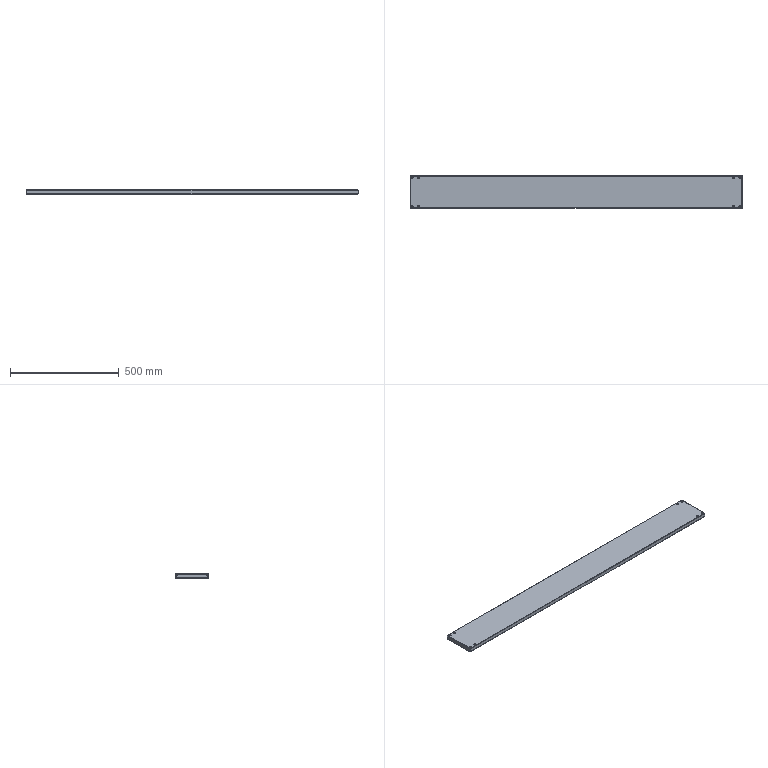Part | SolidWorks | features BaseBody 9 | 9 solids | 170 faces | box 1530 x 150 x 20 mm | volume 628139 mm3 | plane 114 | cylinder 48 | spline 8 | commonest cylinder face diameters 5 x16 8 x16 0.4 x8 4.4 x8